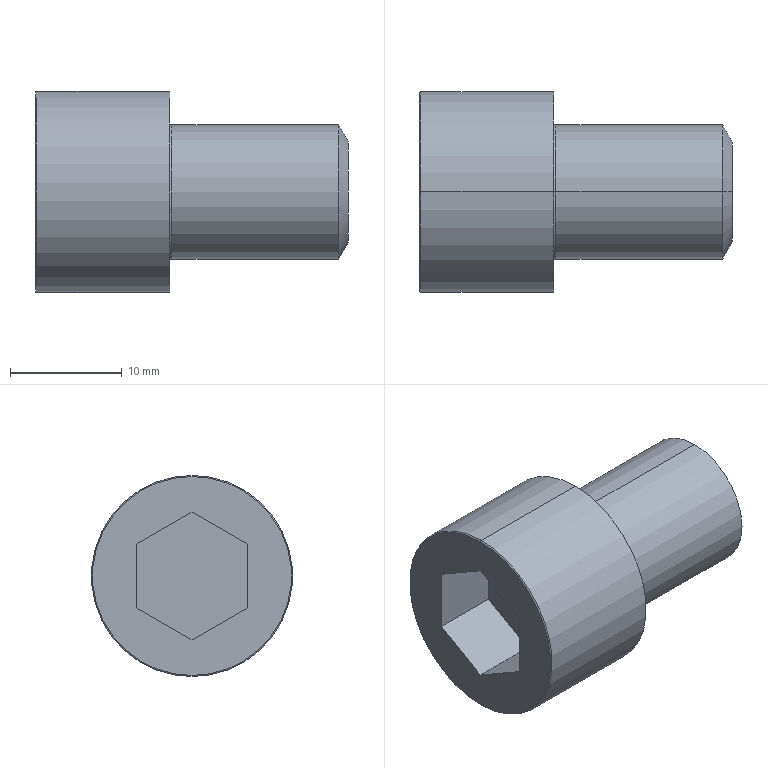Part | STEP file | 1 solid | 20 faces | box 28 x 18 x 18 mm | volume 4331 mm3 | plane 10 | torus 4 | cylinder 4 | cone 2 | commonest cylinder face diameters 12 x2 18 x2
STEP:
#1=CARTESIAN_POINT('',(0.,0.,8.9));
#2=VERTEX_POINT('',#1);
#3=CARTESIAN_POINT('',(0.,0.,-8.9));
#4=VERTEX_POINT('',#3);
#5=CARTESIAN_POINT('',(0.,0.,0.));
#6=DIRECTION('',(-1.,0.,0.));
#7=DIRECTION('',(0.,0.,-1.));
#8=AXIS2_PLACEMENT_3D('',#5,#6,#7);
#9=CIRCLE('',#8,8.9);
#10=EDGE_CURVE('',#2,#4,#9,.T.);
#11=ORIENTED_EDGE('',*,*,#10,.F.);
#12=CARTESIAN_POINT('',(0.1,0.,9.));
#13=VERTEX_POINT('',#12);
#14=CARTESIAN_POINT('',(0.1,0.,8.9));
#15=DIRECTION('',(0.,1.,0.));
#16=DIRECTION('',(0.,0.,1.));
#17=AXIS2_PLACEMENT_3D('',#14,#15,#16);
#18=CIRCLE('',#17,0.1);
#19=EDGE_CURVE('',#2,#13,#18,.T.);
#20=ORIENTED_EDGE('',*,*,#19,.T.);
#21=CARTESIAN_POINT('',(0.1,0.,-9.));
#22=VERTEX_POINT('',#21);
#23=CARTESIAN_POINT('',(0.1,0.,0.));
#24=DIRECTION('',(1.,0.,0.));
#25=DIRECTION('',(0.,0.,-1.));
#26=AXIS2_PLACEMENT_3D('',#23,#24,#25);
#27=CIRCLE('',#26,9.);
#28=EDGE_CURVE('',#22,#13,#27,.T.);
#29=ORIENTED_EDGE('',*,*,#28,.F.);
#30=CARTESIAN_POINT('',(0.1,0.,-8.9));
#31=DIRECTION('',(0.,-1.,0.));
#32=DIRECTION('',(0.,0.,-1.));
#33=AXIS2_PLACEMENT_3D('',#30,#31,#32);
#34=CIRCLE('',#33,0.1);
#35=EDGE_CURVE('',#4,#22,#34,.T.);
#36=ORIENTED_EDGE('',*,*,#35,.F.);
#37=EDGE_LOOP('',(#11,#20,#29,#36));
#38=FACE_OUTER_BOUND('',#37,.T.);
#39=CARTESIAN_POINT('',(0.1,0.,0.));
#40=DIRECTION('',(1.,0.,0.));
#41=DIRECTION('',(0.,0.,-1.));
#42=AXIS2_PLACEMENT_3D('',#39,#40,#41);
#43=TOROIDAL_SURFACE('',#42,8.9,0.1);
#44=ADVANCED_FACE('',(#38),#43,.T.);
#45=CARTESIAN_POINT('',(28.,0.,4.484));
#46=VERTEX_POINT('',#45);
#47=CARTESIAN_POINT('',(28.,0.,-4.484));
#48=VERTEX_POINT('',#47);
#49=CARTESIAN_POINT('',(28.,0.,0.));
#50=DIRECTION('',(-1.,0.,0.));
#51=DIRECTION('',(0.,0.,1.));
#52=AXIS2_PLACEMENT_3D('',#49,#50,#51);
#53=CIRCLE('',#52,4.484);
#54=EDGE_CURVE('',#46,#48,#53,.T.);
#55=ORIENTED_EDGE('',*,*,#54,.T.);
#56=CARTESIAN_POINT('',(27.125,0.,-6.));
#57=VERTEX_POINT('',#56);
#58=CARTESIAN_POINT('',(27.125,0.,-6.));
#59=DIRECTION('',(-0.5,0.,-0.866));
#60=VECTOR('',#59,1000.);
#61=LINE('',#58,#60);
#62=EDGE_CURVE('',#48,#57,#61,.T.);
#63=ORIENTED_EDGE('',*,*,#62,.T.);
#64=CARTESIAN_POINT('',(27.125,0.,6.));
#65=VERTEX_POINT('',#64);
#66=CARTESIAN_POINT('',(27.125,0.,0.));
#67=DIRECTION('',(-1.,0.,0.));
#68=DIRECTION('',(0.,0.,1.));
#69=AXIS2_PLACEMENT_3D('',#66,#67,#68);
#70=CIRCLE('',#69,6.);
#71=EDGE_CURVE('',#65,#57,#70,.T.);
#72=ORIENTED_EDGE('',*,*,#71,.F.);
#73=CARTESIAN_POINT('',(27.125,0.,6.));
#74=DIRECTION('',(-0.5,0.,0.866));
#75=VECTOR('',#74,1000.);
#76=LINE('',#73,#75);
#77=EDGE_CURVE('',#46,#65,#76,.T.);
#78=ORIENTED_EDGE('',*,*,#77,.F.);
#79=EDGE_LOOP('',(#55,#63,#72,#78));
#80=FACE_OUTER_BOUND('',#79,.T.);
#81=CARTESIAN_POINT('',(27.125,0.,0.));
#82=DIRECTION('',(-1.,0.,0.));
#83=DIRECTION('',(0.,0.,1.));
#84=AXIS2_PLACEMENT_3D('',#81,#82,#83);
#85=CONICAL_SURFACE('',#84,6.,1.047);
#86=ADVANCED_FACE('',(#80),#85,.T.);
#87=CARTESIAN_POINT('',(12.,0.,-6.2));
#88=VERTEX_POINT('',#87);
#89=CARTESIAN_POINT('',(12.,0.,6.2));
#90=VERTEX_POINT('',#89);
#91=CARTESIAN_POINT('',(12.,0.,0.));
#92=DIRECTION('',(-1.,0.,0.));
#93=DIRECTION('',(0.,0.,1.));
#94=AXIS2_PLACEMENT_3D('',#91,#92,#93);
#95=CIRCLE('',#94,6.2);
#96=EDGE_CURVE('',#88,#90,#95,.T.);
#97=ORIENTED_EDGE('',*,*,#96,.F.);
#98=CARTESIAN_POINT('',(12.2,0.,-6.));
#99=VERTEX_POINT('',#98);
#100=CARTESIAN_POINT('',(12.2,0.,-6.2));
#101=DIRECTION('',(0.,1.,0.));
#102=DIRECTION('',(0.,0.,1.));
#103=AXIS2_PLACEMENT_3D('',#100,#101,#102);
#104=CIRCLE('',#103,0.2);
#105=EDGE_CURVE('',#88,#99,#104,.T.);
#106=ORIENTED_EDGE('',*,*,#105,.T.);
#107=CARTESIAN_POINT('',(12.2,0.,6.));
#108=VERTEX_POINT('',#107);
#109=CARTESIAN_POINT('',(12.2,0.,0.));
#110=DIRECTION('',(-1.,0.,0.));
#111=DIRECTION('',(0.,0.,1.));
#112=AXIS2_PLACEMENT_3D('',#109,#110,#111);
#113=CIRCLE('',#112,6.);
#114=EDGE_CURVE('',#99,#108,#113,.T.);
#115=ORIENTED_EDGE('',*,*,#114,.T.);
#116=CARTESIAN_POINT('',(12.2,0.,6.2));
#117=DIRECTION('',(0.,-1.,0.));
#118=DIRECTION('',(0.,0.,-1.));
#119=AXIS2_PLACEMENT_3D('',#116,#117,#118);
#120=CIRCLE('',#119,0.2);
#121=EDGE_CURVE('',#90,#108,#120,.T.);
#122=ORIENTED_EDGE('',*,*,#121,.F.);
#123=EDGE_LOOP('',(#97,#106,#115,#122));
#124=FACE_OUTER_BOUND('',#123,.T.);
#125=CARTESIAN_POINT('',(12.2,0.,0.));
#126=DIRECTION('',(-1.,0.,0.));
#127=DIRECTION('',(0.,0.,1.));
#128=AXIS2_PLACEMENT_3D('',#125,#126,#127);
#129=TOROIDAL_SURFACE('',#128,6.2,0.2);
#130=ADVANCED_FACE('',(#124),#129,.F.);
#131=CARTESIAN_POINT('',(12.,0.,9.));
#132=VERTEX_POINT('',#131);
#133=CARTESIAN_POINT('',(12.,0.,-9.));
#134=VERTEX_POINT('',#133);
#135=CARTESIAN_POINT('',(12.,0.,0.));
#136=DIRECTION('',(-1.,0.,0.));
#137=DIRECTION('',(0.,0.,1.));
#138=AXIS2_PLACEMENT_3D('',#135,#136,#137);
#139=CIRCLE('',#138,9.);
#140=EDGE_CURVE('',#132,#134,#139,.T.);
#141=ORIENTED_EDGE('',*,*,#140,.T.);
#142=CARTESIAN_POINT('',(0.,0.,-9.));
#143=DIRECTION('',(-1.,0.,0.));
#144=VECTOR('',#143,1000.);
#145=LINE('',#142,#144);
#146=EDGE_CURVE('',#134,#22,#145,.T.);
#147=ORIENTED_EDGE('',*,*,#146,.T.);
#148=ORIENTED_EDGE('',*,*,#28,.T.);
#149=CARTESIAN_POINT('',(0.,0.,9.));
#150=DIRECTION('',(-1.,0.,0.));
#151=VECTOR('',#150,1000.);
#152=LINE('',#149,#151);
#153=EDGE_CURVE('',#132,#13,#152,.T.);
#154=ORIENTED_EDGE('',*,*,#153,.F.);
#155=EDGE_LOOP('',(#141,#147,#148,#154));
#156=FACE_OUTER_BOUND('',#155,.T.);
#157=CARTESIAN_POINT('',(0.,0.,0.));
#158=DIRECTION('',(-1.,0.,0.));
#159=DIRECTION('',(0.,0.,1.));
#160=AXIS2_PLACEMENT_3D('',#157,#158,#159);
#161=CYLINDRICAL_SURFACE('',#160,9.);
#162=ADVANCED_FACE('',(#156),#161,.T.);
#163=ORIENTED_EDGE('',*,*,#71,.T.);
#164=CARTESIAN_POINT('',(0.,0.,-6.));
#165=DIRECTION('',(-1.,0.,0.));
#166=VECTOR('',#165,1000.);
#167=LINE('',#164,#166);
#168=EDGE_CURVE('',#57,#99,#167,.T.);
#169=ORIENTED_EDGE('',*,*,#168,.T.);
#170=CARTESIAN_POINT('',(12.2,0.,0.));
#171=DIRECTION('',(-1.,0.,0.));
#172=DIRECTION('',(0.,0.,1.));
#173=AXIS2_PLACEMENT_3D('',#170,#171,#172);
#174=CIRCLE('',#173,6.);
#175=EDGE_CURVE('',#108,#99,#174,.T.);
#176=ORIENTED_EDGE('',*,*,#175,.F.);
#177=CARTESIAN_POINT('',(0.,0.,6.));
#178=DIRECTION('',(-1.,0.,0.));
#179=VECTOR('',#178,1000.);
#180=LINE('',#177,#179);
#181=EDGE_CURVE('',#65,#108,#180,.T.);
#182=ORIENTED_EDGE('',*,*,#181,.F.);
#183=EDGE_LOOP('',(#163,#169,#176,#182));
#184=FACE_OUTER_BOUND('',#183,.T.);
#185=CARTESIAN_POINT('',(0.,0.,0.));
#186=DIRECTION('',(-1.,0.,0.));
#187=DIRECTION('',(0.,0.,1.));
#188=AXIS2_PLACEMENT_3D('',#185,#186,#187);
#189=CYLINDRICAL_SURFACE('',#188,6.);
#190=ADVANCED_FACE('',(#184),#189,.T.);
#191=ORIENTED_EDGE('',*,*,#168,.F.);
#192=CARTESIAN_POINT('',(27.125,0.,0.));
#193=DIRECTION('',(-1.,0.,0.));
#194=DIRECTION('',(0.,0.,1.));
#195=AXIS2_PLACEMENT_3D('',#192,#193,#194);
#196=CIRCLE('',#195,6.);
#197=EDGE_CURVE('',#57,#65,#196,.T.);
#198=ORIENTED_EDGE('',*,*,#197,.T.);
#199=ORIENTED_EDGE('',*,*,#181,.T.);
#200=ORIENTED_EDGE('',*,*,#114,.F.);
#201=EDGE_LOOP('',(#191,#198,#199,#200));
#202=FACE_OUTER_BOUND('',#201,.T.);
#203=CARTESIAN_POINT('',(0.,0.,0.));
#204=DIRECTION('',(-1.,0.,0.));
#205=DIRECTION('',(0.,0.,1.));
#206=AXIS2_PLACEMENT_3D('',#203,#204,#205);
#207=CYLINDRICAL_SURFACE('',#206,6.);
#208=ADVANCED_FACE('',(#202),#207,.T.);
#209=CARTESIAN_POINT('',(0.,0.,0.));
#210=DIRECTION('',(-1.,0.,0.));
#211=DIRECTION('',(0.,0.,-1.));
#212=AXIS2_PLACEMENT_3D('',#209,#210,#211);
#213=CIRCLE('',#212,8.9);
#214=EDGE_CURVE('',#4,#2,#213,.T.);
#215=ORIENTED_EDGE('',*,*,#214,.T.);
#216=ORIENTED_EDGE('',*,*,#10,.T.);
#217=EDGE_LOOP('',(#215,#216));
#218=FACE_OUTER_BOUND('',#217,.T.);
#219=CARTESIAN_POINT('',(0.,0.,5.715));
#220=VERTEX_POINT('',#219);
#221=CARTESIAN_POINT('',(0.,4.949,2.857));
#222=VERTEX_POINT('',#221);
#223=CARTESIAN_POINT('',(0.,0.,5.715));
#224=DIRECTION('',(0.,0.866,-0.5));
#225=VECTOR('',#224,1000.);
#226=LINE('',#223,#225);
#227=EDGE_CURVE('',#220,#222,#226,.T.);
#228=ORIENTED_EDGE('',*,*,#227,.F.);
#229=CARTESIAN_POINT('',(0.,-4.949,2.858));
#230=VERTEX_POINT('',#229);
#231=CARTESIAN_POINT('',(0.,-4.949,2.858));
#232=DIRECTION('',(0.,0.866,0.5));
#233=VECTOR('',#232,1000.);
#234=LINE('',#231,#233);
#235=EDGE_CURVE('',#230,#220,#234,.T.);
#236=ORIENTED_EDGE('',*,*,#235,.F.);
#237=CARTESIAN_POINT('',(0.,-4.949,-2.857));
#238=VERTEX_POINT('',#237);
#239=CARTESIAN_POINT('',(0.,-4.949,-2.857));
#240=DIRECTION('',(0.,0.,1.));
#241=VECTOR('',#240,1000.);
#242=LINE('',#239,#241);
#243=EDGE_CURVE('',#238,#230,#242,.T.);
#244=ORIENTED_EDGE('',*,*,#243,.F.);
#245=CARTESIAN_POINT('',(0.,0.,-5.715));
#246=VERTEX_POINT('',#245);
#247=CARTESIAN_POINT('',(0.,0.,-5.715));
#248=DIRECTION('',(0.,-0.866,0.5));
#249=VECTOR('',#248,1000.);
#250=LINE('',#247,#249);
#251=EDGE_CURVE('',#246,#238,#250,.T.);
#252=ORIENTED_EDGE('',*,*,#251,.F.);
#253=CARTESIAN_POINT('',(0.,4.949,-2.857));
#254=VERTEX_POINT('',#253);
#255=CARTESIAN_POINT('',(0.,4.949,-2.857));
#256=DIRECTION('',(0.,-0.866,-0.5));
#257=VECTOR('',#256,1000.);
#258=LINE('',#255,#257);
#259=EDGE_CURVE('',#254,#246,#258,.T.);
#260=ORIENTED_EDGE('',*,*,#259,.F.);
#261=CARTESIAN_POINT('',(0.,4.949,2.857));
#262=DIRECTION('',(0.,0.,-1.));
#263=VECTOR('',#262,1000.);
#264=LINE('',#261,#263);
#265=EDGE_CURVE('',#222,#254,#264,.T.);
#266=ORIENTED_EDGE('',*,*,#265,.F.);
#267=EDGE_LOOP('',(#228,#236,#244,#252,#260,#266));
#268=FACE_BOUND('',#267,.T.);
#269=CARTESIAN_POINT('',(0.,0.,0.));
#270=DIRECTION('',(1.,0.,0.));
#271=DIRECTION('',(0.,0.,-1.));
#272=AXIS2_PLACEMENT_3D('',#269,#270,#271);
#273=PLANE('',#272);
#274=ADVANCED_FACE('',(#218,#268),#273,.F.);
#275=ORIENTED_EDGE('',*,*,#146,.F.);
#276=CARTESIAN_POINT('',(12.,0.,0.));
#277=DIRECTION('',(-1.,0.,0.));
#278=DIRECTION('',(0.,0.,1.));
#279=AXIS2_PLACEMENT_3D('',#276,#277,#278);
#280=CIRCLE('',#279,9.);
#281=EDGE_CURVE('',#134,#132,#280,.T.);
#282=ORIENTED_EDGE('',*,*,#281,.T.);
#283=ORIENTED_EDGE('',*,*,#153,.T.);
#284=CARTESIAN_POINT('',(0.1,0.,0.));
#285=DIRECTION('',(1.,0.,0.));
#286=DIRECTION('',(0.,0.,-1.));
#287=AXIS2_PLACEMENT_3D('',#284,#285,#286);
#288=CIRCLE('',#287,9.);
#289=EDGE_CURVE('',#13,#22,#288,.T.);
#290=ORIENTED_EDGE('',*,*,#289,.T.);
#291=EDGE_LOOP('',(#275,#282,#283,#290));
#292=FACE_OUTER_BOUND('',#291,.T.);
#293=CARTESIAN_POINT('',(0.,0.,0.));
#294=DIRECTION('',(-1.,0.,0.));
#295=DIRECTION('',(0.,0.,1.));
#296=AXIS2_PLACEMENT_3D('',#293,#294,#295);
#297=CYLINDRICAL_SURFACE('',#296,9.);
#298=ADVANCED_FACE('',(#292),#297,.T.);
#299=ORIENTED_EDGE('',*,*,#140,.F.);
#300=ORIENTED_EDGE('',*,*,#281,.F.);
#301=EDGE_LOOP('',(#299,#300));
#302=FACE_OUTER_BOUND('',#301,.T.);
#303=CARTESIAN_POINT('',(12.,0.,0.));
#304=DIRECTION('',(-1.,0.,0.));
#305=DIRECTION('',(0.,0.,1.));
#306=AXIS2_PLACEMENT_3D('',#303,#304,#305);
#307=CIRCLE('',#306,6.2);
#308=EDGE_CURVE('',#90,#88,#307,.T.);
#309=ORIENTED_EDGE('',*,*,#308,.T.);
#310=ORIENTED_EDGE('',*,*,#96,.T.);
#311=EDGE_LOOP('',(#309,#310));
#312=FACE_BOUND('',#311,.T.);
#313=CARTESIAN_POINT('',(12.,9.,0.));
#314=DIRECTION('',(-1.,0.,0.));
#315=DIRECTION('',(0.,0.,1.));
#316=AXIS2_PLACEMENT_3D('',#313,#314,#315);
#317=PLANE('',#316);
#318=ADVANCED_FACE('',(#302,#312),#317,.F.);
#319=ORIENTED_EDGE('',*,*,#105,.F.);
#320=ORIENTED_EDGE('',*,*,#308,.F.);
#321=ORIENTED_EDGE('',*,*,#121,.T.);
#322=ORIENTED_EDGE('',*,*,#175,.T.);
#323=EDGE_LOOP('',(#319,#320,#321,#322));
#324=FACE_OUTER_BOUND('',#323,.T.);
#325=CARTESIAN_POINT('',(12.2,0.,0.));
#326=DIRECTION('',(-1.,0.,0.));
#327=DIRECTION('',(0.,0.,1.));
#328=AXIS2_PLACEMENT_3D('',#325,#326,#327);
#329=TOROIDAL_SURFACE('',#328,6.2,0.2);
#330=ADVANCED_FACE('',(#324),#329,.F.);
#331=ORIENTED_EDGE('',*,*,#235,.T.);
#332=CARTESIAN_POINT('',(6.,0.,5.715));
#333=VERTEX_POINT('',#332);
#334=CARTESIAN_POINT('',(6.,0.,5.715));
#335=DIRECTION('',(-1.,0.,0.));
#336=VECTOR('',#335,1000.);
#337=LINE('',#334,#336);
#338=EDGE_CURVE('',#333,#220,#337,.T.);
#339=ORIENTED_EDGE('',*,*,#338,.F.);
#340=CARTESIAN_POINT('',(6.,-4.949,2.858));
#341=VERTEX_POINT('',#340);
#342=CARTESIAN_POINT('',(6.,-4.949,2.858));
#343=DIRECTION('',(0.,0.866,0.5));
#344=VECTOR('',#343,1000.);
#345=LINE('',#342,#344);
#346=EDGE_CURVE('',#341,#333,#345,.T.);
#347=ORIENTED_EDGE('',*,*,#346,.F.);
#348=CARTESIAN_POINT('',(6.,-4.949,2.858));
#349=DIRECTION('',(-1.,0.,0.));
#350=VECTOR('',#349,1000.);
#351=LINE('',#348,#350);
#352=EDGE_CURVE('',#341,#230,#351,.T.);
#353=ORIENTED_EDGE('',*,*,#352,.T.);
#354=EDGE_LOOP('',(#331,#339,#347,#353));
#355=FACE_OUTER_BOUND('',#354,.T.);
#356=CARTESIAN_POINT('',(6.,-4.949,2.858));
#357=DIRECTION('',(0.,-0.5,0.866));
#358=DIRECTION('',(0.,-0.866,-0.5));
#359=AXIS2_PLACEMENT_3D('',#356,#357,#358);
#360=PLANE('',#359);
#361=ADVANCED_FACE('',(#355),#360,.F.);
#362=ORIENTED_EDGE('',*,*,#243,.T.);
#363=ORIENTED_EDGE('',*,*,#352,.F.);
#364=CARTESIAN_POINT('',(6.,-4.949,-2.857));
#365=VERTEX_POINT('',#364);
#366=CARTESIAN_POINT('',(6.,-4.949,-2.857));
#367=DIRECTION('',(0.,0.,1.));
#368=VECTOR('',#367,1000.);
#369=LINE('',#366,#368);
#370=EDGE_CURVE('',#365,#341,#369,.T.);
#371=ORIENTED_EDGE('',*,*,#370,.F.);
#372=CARTESIAN_POINT('',(6.,-4.949,-2.857));
#373=DIRECTION('',(-1.,0.,0.));
#374=VECTOR('',#373,1000.);
#375=LINE('',#372,#374);
#376=EDGE_CURVE('',#365,#238,#375,.T.);
#377=ORIENTED_EDGE('',*,*,#376,.T.);
#378=EDGE_LOOP('',(#362,#363,#371,#377));
#379=FACE_OUTER_BOUND('',#378,.T.);
#380=CARTESIAN_POINT('',(6.,-4.949,-2.857));
#381=DIRECTION('',(0.,-1.,0.));
#382=DIRECTION('',(0.,0.,-1.));
#383=AXIS2_PLACEMENT_3D('',#380,#381,#382);
#384=PLANE('',#383);
#385=ADVANCED_FACE('',(#379),#384,.F.);
#386=ORIENTED_EDGE('',*,*,#251,.T.);
#387=ORIENTED_EDGE('',*,*,#376,.F.);
#388=CARTESIAN_POINT('',(6.,0.,-5.715));
#389=VERTEX_POINT('',#388);
#390=CARTESIAN_POINT('',(6.,0.,-5.715));
#391=DIRECTION('',(0.,-0.866,0.5));
#392=VECTOR('',#391,1000.);
#393=LINE('',#390,#392);
#394=EDGE_CURVE('',#389,#365,#393,.T.);
#395=ORIENTED_EDGE('',*,*,#394,.F.);
#396=CARTESIAN_POINT('',(6.,0.,-5.715));
#397=DIRECTION('',(-1.,0.,0.));
#398=VECTOR('',#397,1000.);
#399=LINE('',#396,#398);
#400=EDGE_CURVE('',#389,#246,#399,.T.);
#401=ORIENTED_EDGE('',*,*,#400,.T.);
#402=EDGE_LOOP('',(#386,#387,#395,#401));
#403=FACE_OUTER_BOUND('',#402,.T.);
#404=CARTESIAN_POINT('',(6.,0.,-5.715));
#405=DIRECTION('',(0.,-0.5,-0.866));
#406=DIRECTION('',(0.,0.866,-0.5));
#407=AXIS2_PLACEMENT_3D('',#404,#405,#406);
#408=PLANE('',#407);
#409=ADVANCED_FACE('',(#403),#408,.F.);
#410=ORIENTED_EDGE('',*,*,#259,.T.);
#411=ORIENTED_EDGE('',*,*,#400,.F.);
#412=CARTESIAN_POINT('',(6.,4.949,-2.857));
#413=VERTEX_POINT('',#412);
#414=CARTESIAN_POINT('',(6.,4.949,-2.857));
#415=DIRECTION('',(0.,-0.866,-0.5));
#416=VECTOR('',#415,1000.);
#417=LINE('',#414,#416);
#418=EDGE_CURVE('',#413,#389,#417,.T.);
#419=ORIENTED_EDGE('',*,*,#418,.F.);
#420=CARTESIAN_POINT('',(6.,4.949,-2.857));
#421=DIRECTION('',(-1.,0.,0.));
#422=VECTOR('',#421,1000.);
#423=LINE('',#420,#422);
#424=EDGE_CURVE('',#413,#254,#423,.T.);
#425=ORIENTED_EDGE('',*,*,#424,.T.);
#426=EDGE_LOOP('',(#410,#411,#419,#425));
#427=FACE_OUTER_BOUND('',#426,.T.);
#428=CARTESIAN_POINT('',(6.,4.949,-2.857));
#429=DIRECTION('',(0.,0.5,-0.866));
#430=DIRECTION('',(0.,0.866,0.5));
#431=AXIS2_PLACEMENT_3D('',#428,#429,#430);
#432=PLANE('',#431);
#433=ADVANCED_FACE('',(#427),#432,.F.);
#434=ORIENTED_EDGE('',*,*,#265,.T.);
#435=ORIENTED_EDGE('',*,*,#424,.F.);
#436=CARTESIAN_POINT('',(6.,4.949,2.857));
#437=VERTEX_POINT('',#436);
#438=CARTESIAN_POINT('',(6.,4.949,2.857));
#439=DIRECTION('',(0.,0.,-1.));
#440=VECTOR('',#439,1000.);
#441=LINE('',#438,#440);
#442=EDGE_CURVE('',#437,#413,#441,.T.);
#443=ORIENTED_EDGE('',*,*,#442,.F.);
#444=CARTESIAN_POINT('',(6.,4.949,2.857));
#445=DIRECTION('',(-1.,0.,0.));
#446=VECTOR('',#445,1000.);
#447=LINE('',#444,#446);
#448=EDGE_CURVE('',#437,#222,#447,.T.);
#449=ORIENTED_EDGE('',*,*,#448,.T.);
#450=EDGE_LOOP('',(#434,#435,#443,#449));
#451=FACE_OUTER_BOUND('',#450,.T.);
#452=CARTESIAN_POINT('',(6.,4.949,2.857));
#453=DIRECTION('',(0.,1.,0.));
#454=DIRECTION('',(0.,0.,1.));
#455=AXIS2_PLACEMENT_3D('',#452,#453,#454);
#456=PLANE('',#455);
#457=ADVANCED_FACE('',(#451),#456,.F.);
#458=ORIENTED_EDGE('',*,*,#227,.T.);
#459=ORIENTED_EDGE('',*,*,#448,.F.);
#460=CARTESIAN_POINT('',(6.,0.,5.715));
#461=DIRECTION('',(0.,0.866,-0.5));
#462=VECTOR('',#461,1000.);
#463=LINE('',#460,#462);
#464=EDGE_CURVE('',#333,#437,#463,.T.);
#465=ORIENTED_EDGE('',*,*,#464,.F.);
#466=ORIENTED_EDGE('',*,*,#338,.T.);
#467=EDGE_LOOP('',(#458,#459,#465,#466));
#468=FACE_OUTER_BOUND('',#467,.T.);
#469=CARTESIAN_POINT('',(6.,0.,5.715));
#470=DIRECTION('',(0.,0.5,0.866));
#471=DIRECTION('',(0.,-0.866,0.5));
#472=AXIS2_PLACEMENT_3D('',#469,#470,#471);
#473=PLANE('',#472);
#474=ADVANCED_FACE('',(#468),#473,.F.);
#475=ORIENTED_EDGE('',*,*,#346,.T.);
#476=ORIENTED_EDGE('',*,*,#464,.T.);
#477=ORIENTED_EDGE('',*,*,#442,.T.);
#478=ORIENTED_EDGE('',*,*,#418,.T.);
#479=ORIENTED_EDGE('',*,*,#394,.T.);
#480=ORIENTED_EDGE('',*,*,#370,.T.);
#481=EDGE_LOOP('',(#475,#476,#477,#478,#479,#480));
#482=FACE_OUTER_BOUND('',#481,.T.);
#483=CARTESIAN_POINT('',(6.,-4.949,2.858));
#484=DIRECTION('',(1.,0.,0.));
#485=DIRECTION('',(0.,0.,-1.));
#486=AXIS2_PLACEMENT_3D('',#483,#484,#485);
#487=PLANE('',#486);
#488=ADVANCED_FACE('',(#482),#487,.F.);
#489=ORIENTED_EDGE('',*,*,#62,.F.);
#490=CARTESIAN_POINT('',(28.,0.,0.));
#491=DIRECTION('',(-1.,0.,0.));
#492=DIRECTION('',(0.,0.,1.));
#493=AXIS2_PLACEMENT_3D('',#490,#491,#492);
#494=CIRCLE('',#493,4.484);
#495=EDGE_CURVE('',#48,#46,#494,.T.);
#496=ORIENTED_EDGE('',*,*,#495,.T.);
#497=ORIENTED_EDGE('',*,*,#77,.T.);
#498=ORIENTED_EDGE('',*,*,#197,.F.);
#499=EDGE_LOOP('',(#489,#496,#497,#498));
#500=FACE_OUTER_BOUND('',#499,.T.);
#501=CARTESIAN_POINT('',(27.125,0.,0.));
#502=DIRECTION('',(-1.,0.,0.));
#503=DIRECTION('',(0.,0.,1.));
#504=AXIS2_PLACEMENT_3D('',#501,#502,#503);
#505=CONICAL_SURFACE('',#504,6.,1.047);
#506=ADVANCED_FACE('',(#500),#505,.T.);
#507=ORIENTED_EDGE('',*,*,#54,.F.);
#508=ORIENTED_EDGE('',*,*,#495,.F.);
#509=EDGE_LOOP('',(#507,#508));
#510=FACE_OUTER_BOUND('',#509,.T.);
#511=CARTESIAN_POINT('',(28.,6.,0.));
#512=DIRECTION('',(-1.,0.,0.));
#513=DIRECTION('',(0.,0.,1.));
#514=AXIS2_PLACEMENT_3D('',#511,#512,#513);
#515=PLANE('',#514);
#516=ADVANCED_FACE('',(#510),#515,.F.);
#517=ORIENTED_EDGE('',*,*,#19,.F.);
#518=ORIENTED_EDGE('',*,*,#214,.F.);
#519=ORIENTED_EDGE('',*,*,#35,.T.);
#520=ORIENTED_EDGE('',*,*,#289,.F.);
#521=EDGE_LOOP('',(#517,#518,#519,#520));
#522=FACE_OUTER_BOUND('',#521,.T.);
#523=CARTESIAN_POINT('',(0.1,0.,0.));
#524=DIRECTION('',(1.,0.,0.));
#525=DIRECTION('',(0.,0.,-1.));
#526=AXIS2_PLACEMENT_3D('',#523,#524,#525);
#527=TOROIDAL_SURFACE('',#526,8.9,0.1);
#528=ADVANCED_FACE('',(#522),#527,.T.);
#529=CLOSED_SHELL('',(#44,#86,#130,#162,#190,#208,#274,#298,#318,#330,#361,#385,#409,#433,#457,#474,#488,#506,#516,#528));
#530=MANIFOLD_SOLID_BREP('',#529);
#531=CARTESIAN_POINT('',(0.,0.,0.));
#532=DIRECTION('',(0.,0.,1.));
#533=DIRECTION('',(1.,0.,0.));
#534=AXIS2_PLACEMENT_3D('',#531,#532,#533);
#535=(LENGTH_UNIT()NAMED_UNIT(*)SI_UNIT(.MILLI.,.METRE.));
#536=UNCERTAINTY_MEASURE_WITH_UNIT(LENGTH_MEASURE(0.00001),#535,'','');
#537=(NAMED_UNIT(*)PLANE_ANGLE_UNIT()SI_UNIT($,.RADIAN.));
#538=(NAMED_UNIT(*)SI_UNIT($,.STERADIAN.)SOLID_ANGLE_UNIT());
#539=(GEOMETRIC_REPRESENTATION_CONTEXT(3)GLOBAL_UNCERTAINTY_ASSIGNED_CONTEXT((#536))GLOBAL_UNIT_ASSIGNED_CONTEXT((#535,#537,#538))REPRESENTATION_CONTEXT('',''));
#540=ADVANCED_BREP_SHAPE_REPRESENTATION('',(#530,#534),#539);